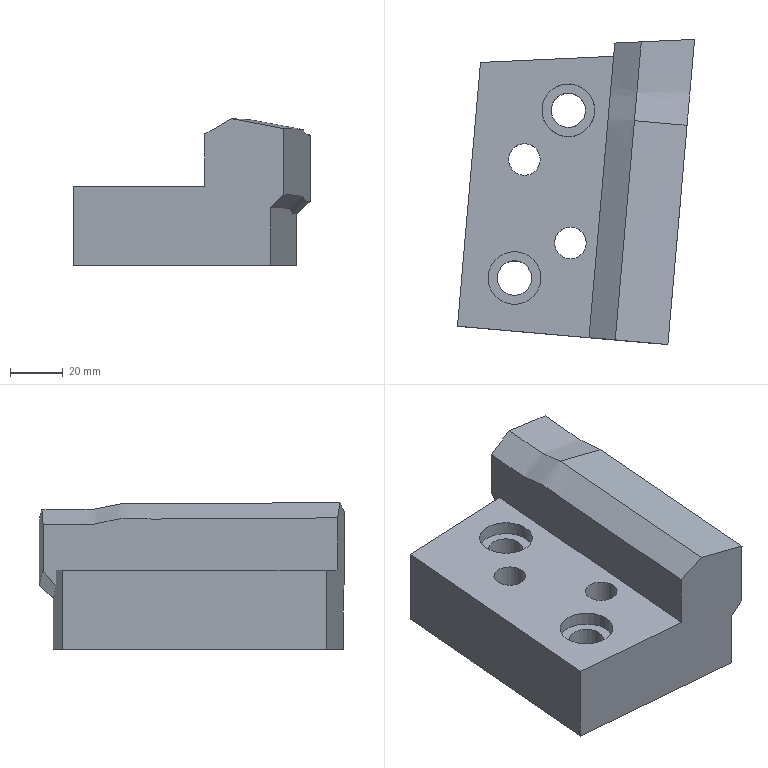Part | NX | features solid 2 | 1 solid | 22 faces | box 89.803 x 115.535 x 55.572 mm | volume 302026 mm3 | plane 9 | spline 7 | cylinder 6 | commonest cylinder face diameters 12 x2 13 x2 20 x2